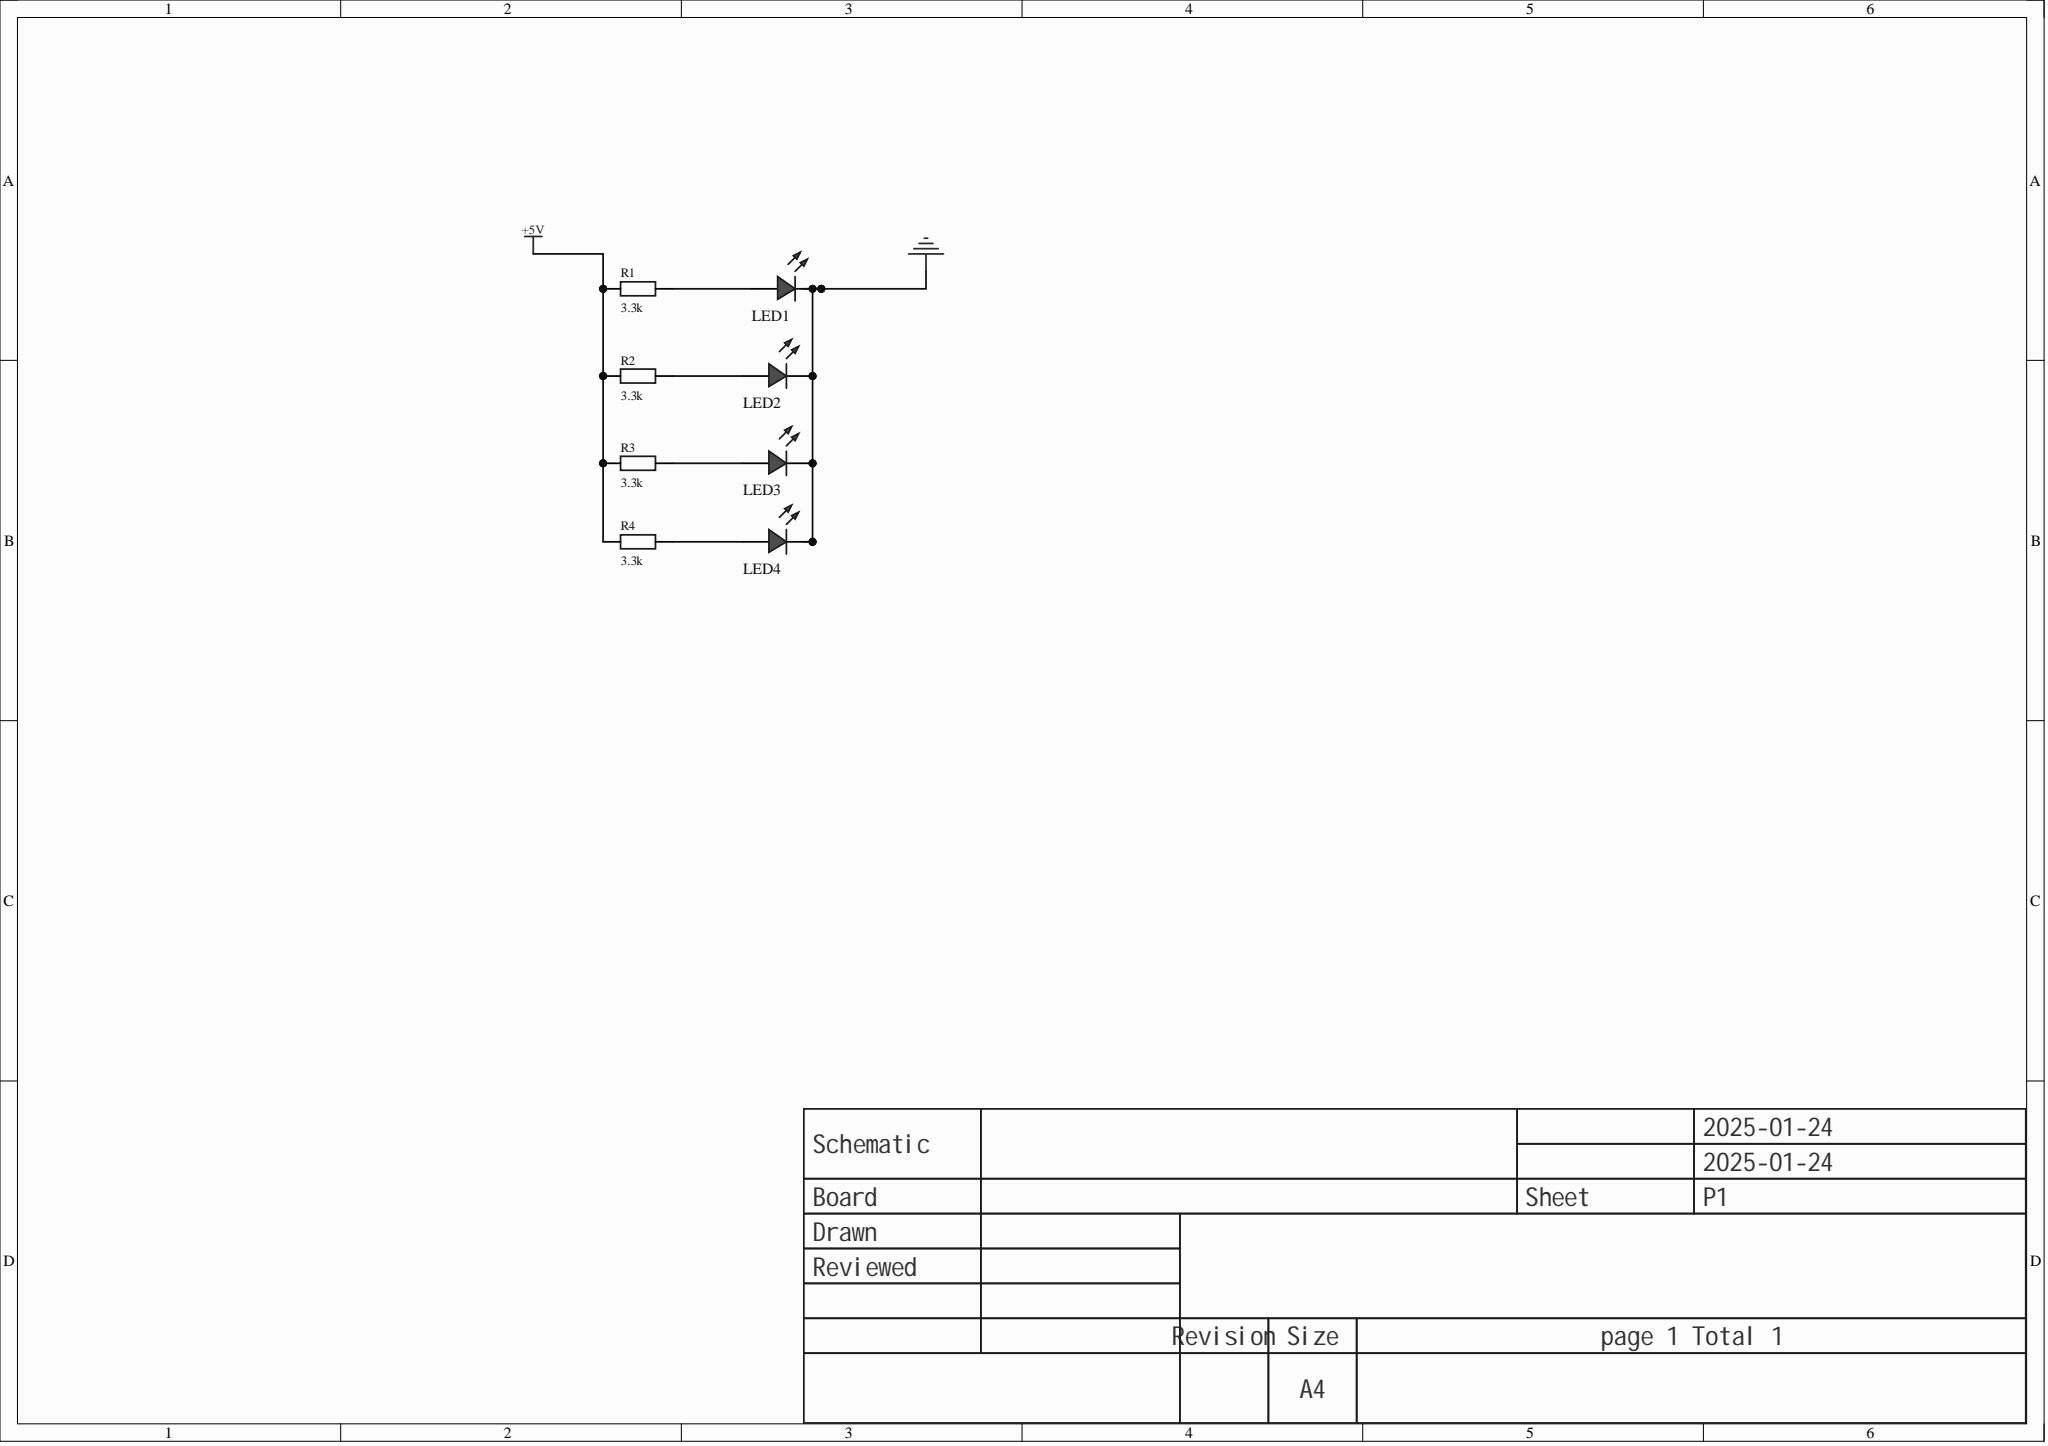Circuit board | Altium Designer | 8 parts | 6 nets
Bill of materials:
Comment,Description,Designator,Footprint,LibRef,Quantity
"","","LED1, LED2, LED3, LED4","LED_0603","LED_0603-R","4"
"3.3k","","R1, R2, R3, R4","R0603","Res_0603","4"
Netlist (Protel format):
[
LED1
LED_0603




]
[
LED2
LED_0603




]
[
LED3
LED_0603




]
[
LED4
LED_0603




]
[
R1
R0603
3.3k



]
[
R2
R0603
3.3k



]
[
R3
R0603
3.3k



]
[
R4
R0603
3.3k



]
(
NetLED4_2
LED4-2
R4-2
)
(
NetLED3_2
LED3-2
R3-2
)
(
NetLED2_2
LED2-2
R2-2
)
(
NetLED1_2
LED1-2
R1-2
)
(
GND
LED1-1
LED2-1
LED3-1
LED4-1
)
(
+5V
R1-1
R2-1
R3-1
R4-1
)